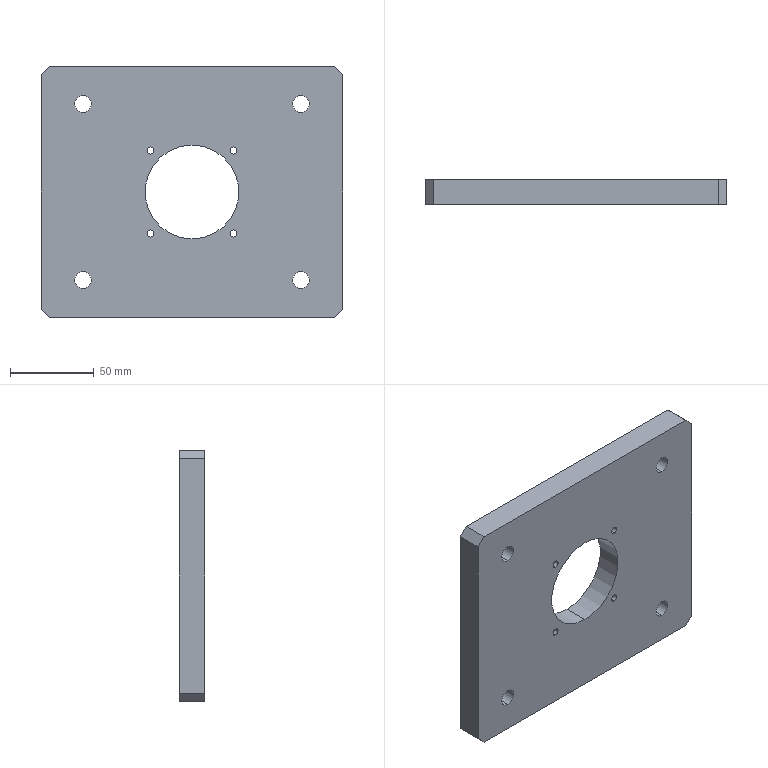Part | STEP file | PN_0020 Motor Plate_Default | 1 solid | 28 faces | box 180 x 15 x 150 mm | volume 361761 mm3 | cylinder 18 | plane 10 | commonest cylinder face diameters 4.2 x8 10 x8 56 x2